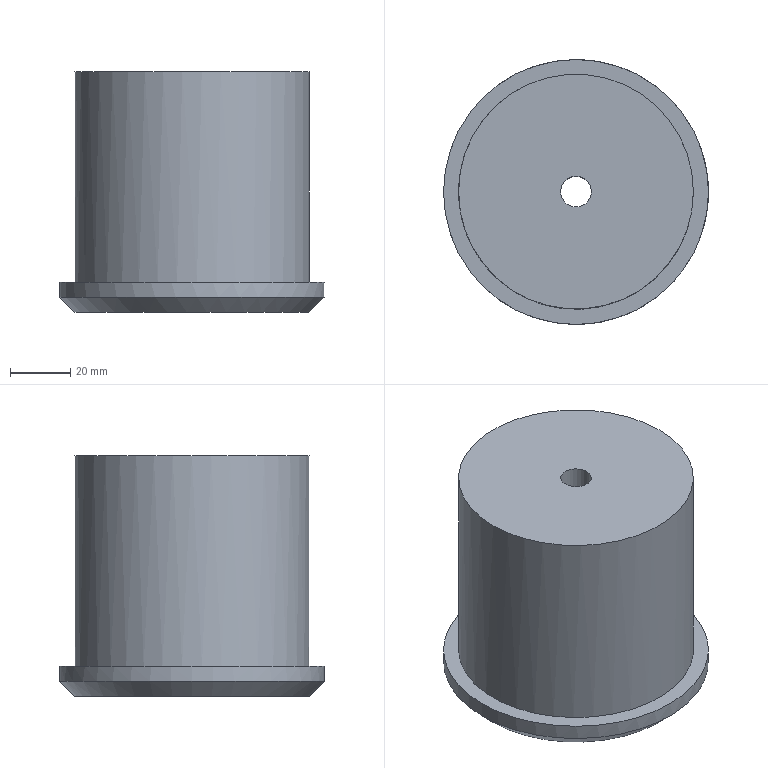Part | STEP file | lll_id810_x_t | 1 solid | 9 faces | box 88 x 88 x 80 mm | volume 376796 mm3 | plane 4 | cylinder 4 | cone 1 | commonest cylinder face diameters 10.2 x1 18.008 x1 78 x1 88 x1
STEP:
#1=CARTESIAN_POINT('',(413.435,500.,-327.5));
#2=VERTEX_POINT('',#1);
#3=CARTESIAN_POINT('',(452.435,500.,-327.5));
#4=DIRECTION('',(0.,0.,-1.));
#5=DIRECTION('',(-1.,0.,0.));
#6=AXIS2_PLACEMENT_3D('',#3,#4,#5);
#7=CIRCLE('',#6,39.);
#8=EDGE_CURVE('',#2,#2,#7,.T.);
#9=ORIENTED_EDGE('',*,*,#8,.F.);
#10=EDGE_LOOP('',(#9));
#11=FACE_BOUND('',#10,.T.);
#12=CARTESIAN_POINT('',(457.535,500.,-327.5));
#13=VERTEX_POINT('',#12);
#14=CARTESIAN_POINT('',(452.435,500.,-327.5));
#15=DIRECTION('',(0.,0.,-1.));
#16=DIRECTION('',(1.,0.,0.));
#17=AXIS2_PLACEMENT_3D('',#14,#15,#16);
#18=CIRCLE('',#17,5.1);
#19=EDGE_CURVE('',#13,#13,#18,.T.);
#20=ORIENTED_EDGE('',*,*,#19,.T.);
#21=EDGE_LOOP('',(#20));
#22=FACE_BOUND('',#21,.T.);
#23=CARTESIAN_POINT('',(452.435,500.,-327.5));
#24=DIRECTION('',(0.,0.,1.));
#25=DIRECTION('',(-1.,0.,0.));
#26=AXIS2_PLACEMENT_3D('',#23,#24,#25);
#27=PLANE('',#26);
#28=ADVANCED_FACE('',(#11,#22),#27,.T.);
#29=CARTESIAN_POINT('',(413.435,500.,-407.5));
#30=VERTEX_POINT('',#29);
#31=CARTESIAN_POINT('',(452.435,500.,-407.5));
#32=DIRECTION('',(0.,0.,-1.));
#33=DIRECTION('',(-1.,0.,0.));
#34=AXIS2_PLACEMENT_3D('',#31,#32,#33);
#35=CIRCLE('',#34,39.);
#36=EDGE_CURVE('',#30,#30,#35,.T.);
#37=ORIENTED_EDGE('',*,*,#36,.T.);
#38=EDGE_LOOP('',(#37));
#39=FACE_BOUND('',#38,.T.);
#40=CARTESIAN_POINT('',(461.439,500.,-407.5));
#41=VERTEX_POINT('',#40);
#42=CARTESIAN_POINT('',(452.435,500.,-407.5));
#43=DIRECTION('',(0.,0.,1.));
#44=DIRECTION('',(1.,0.,0.));
#45=AXIS2_PLACEMENT_3D('',#42,#43,#44);
#46=CIRCLE('',#45,9.004);
#47=EDGE_CURVE('',#41,#41,#46,.T.);
#48=ORIENTED_EDGE('',*,*,#47,.T.);
#49=EDGE_LOOP('',(#48));
#50=FACE_BOUND('',#49,.T.);
#51=CARTESIAN_POINT('',(452.435,500.,-407.5));
#52=DIRECTION('',(0.,0.,-1.));
#53=DIRECTION('',(1.,0.,0.));
#54=AXIS2_PLACEMENT_3D('',#51,#52,#53);
#55=PLANE('',#54);
#56=ADVANCED_FACE('',(#39,#50),#55,.T.);
#57=CARTESIAN_POINT('',(491.435,500.,-397.5));
#58=VERTEX_POINT('',#57);
#59=CARTESIAN_POINT('',(452.435,500.,-397.5));
#60=DIRECTION('',(0.,0.,-1.));
#61=DIRECTION('',(1.,0.,0.));
#62=AXIS2_PLACEMENT_3D('',#59,#60,#61);
#63=CIRCLE('',#62,39.);
#64=EDGE_CURVE('',#58,#58,#63,.T.);
#65=ORIENTED_EDGE('',*,*,#64,.F.);
#66=EDGE_LOOP('',(#65));
#67=FACE_BOUND('',#66,.T.);
#68=ORIENTED_EDGE('',*,*,#8,.T.);
#69=EDGE_LOOP('',(#68));
#70=FACE_BOUND('',#69,.T.);
#71=CARTESIAN_POINT('',(452.435,500.,-327.5));
#72=DIRECTION('',(0.,0.,-1.));
#73=DIRECTION('',(1.,0.,0.));
#74=AXIS2_PLACEMENT_3D('',#71,#72,#73);
#75=CYLINDRICAL_SURFACE('',#74,39.);
#76=ADVANCED_FACE('',(#67,#70),#75,.T.);
#77=ORIENTED_EDGE('',*,*,#64,.T.);
#78=EDGE_LOOP('',(#77));
#79=FACE_BOUND('',#78,.T.);
#80=CARTESIAN_POINT('',(496.435,500.,-397.5));
#81=VERTEX_POINT('',#80);
#82=CARTESIAN_POINT('',(452.435,500.,-397.5));
#83=DIRECTION('',(0.,0.,-1.));
#84=DIRECTION('',(1.,0.,0.));
#85=AXIS2_PLACEMENT_3D('',#82,#83,#84);
#86=CIRCLE('',#85,44.);
#87=EDGE_CURVE('',#81,#81,#86,.T.);
#88=ORIENTED_EDGE('',*,*,#87,.F.);
#89=EDGE_LOOP('',(#88));
#90=FACE_BOUND('',#89,.T.);
#91=CARTESIAN_POINT('',(452.435,500.,-397.5));
#92=DIRECTION('',(0.,0.,1.));
#93=DIRECTION('',(-1.,0.,0.));
#94=AXIS2_PLACEMENT_3D('',#91,#92,#93);
#95=PLANE('',#94);
#96=ADVANCED_FACE('',(#79,#90),#95,.T.);
#97=CARTESIAN_POINT('',(408.435,500.,-402.5));
#98=VERTEX_POINT('',#97);
#99=CARTESIAN_POINT('',(452.435,500.,-402.5));
#100=DIRECTION('',(0.,0.,1.));
#101=DIRECTION('',(-1.,0.,0.));
#102=AXIS2_PLACEMENT_3D('',#99,#100,#101);
#103=CIRCLE('',#102,44.);
#104=EDGE_CURVE('',#98,#98,#103,.T.);
#105=ORIENTED_EDGE('',*,*,#104,.T.);
#106=EDGE_LOOP('',(#105));
#107=FACE_BOUND('',#106,.T.);
#108=ORIENTED_EDGE('',*,*,#87,.T.);
#109=EDGE_LOOP('',(#108));
#110=FACE_BOUND('',#109,.T.);
#111=CARTESIAN_POINT('',(452.435,500.,-407.5));
#112=DIRECTION('',(0.,0.,1.));
#113=DIRECTION('',(-1.,0.,0.));
#114=AXIS2_PLACEMENT_3D('',#111,#112,#113);
#115=CYLINDRICAL_SURFACE('',#114,44.);
#116=ADVANCED_FACE('',(#107,#110),#115,.T.);
#117=ORIENTED_EDGE('',*,*,#36,.F.);
#118=EDGE_LOOP('',(#117));
#119=FACE_BOUND('',#118,.T.);
#120=ORIENTED_EDGE('',*,*,#104,.F.);
#121=EDGE_LOOP('',(#120));
#122=FACE_BOUND('',#121,.T.);
#123=CARTESIAN_POINT('',(452.435,500.,-402.5));
#124=DIRECTION('',(0.,0.,1.));
#125=DIRECTION('',(-1.,0.,0.));
#126=AXIS2_PLACEMENT_3D('',#123,#124,#125);
#127=CONICAL_SURFACE('',#126,44.,45.);
#128=ADVANCED_FACE('',(#119,#122),#127,.T.);
#129=CARTESIAN_POINT('',(457.535,500.,-357.5));
#130=VERTEX_POINT('',#129);
#131=CARTESIAN_POINT('',(452.435,500.,-357.5));
#132=DIRECTION('',(0.,0.,1.));
#133=DIRECTION('',(1.,0.,0.));
#134=AXIS2_PLACEMENT_3D('',#131,#132,#133);
#135=CIRCLE('',#134,5.1);
#136=EDGE_CURVE('',#130,#130,#135,.T.);
#137=ORIENTED_EDGE('',*,*,#136,.F.);
#138=EDGE_LOOP('',(#137));
#139=FACE_BOUND('',#138,.T.);
#140=ORIENTED_EDGE('',*,*,#19,.F.);
#141=EDGE_LOOP('',(#140));
#142=FACE_BOUND('',#141,.T.);
#143=CARTESIAN_POINT('',(452.435,500.,-407.5));
#144=DIRECTION('',(0.,0.,1.));
#145=DIRECTION('',(-1.,0.,0.));
#146=AXIS2_PLACEMENT_3D('',#143,#144,#145);
#147=CYLINDRICAL_SURFACE('',#146,5.1);
#148=ADVANCED_FACE('',(#139,#142),#147,.F.);
#149=ORIENTED_EDGE('',*,*,#136,.T.);
#150=EDGE_LOOP('',(#149));
#151=FACE_BOUND('',#150,.T.);
#152=CARTESIAN_POINT('',(461.439,500.,-357.5));
#153=VERTEX_POINT('',#152);
#154=CARTESIAN_POINT('',(452.435,500.,-357.5));
#155=DIRECTION('',(0.,0.,1.));
#156=DIRECTION('',(1.,0.,0.));
#157=AXIS2_PLACEMENT_3D('',#154,#155,#156);
#158=CIRCLE('',#157,9.004);
#159=EDGE_CURVE('',#153,#153,#158,.T.);
#160=ORIENTED_EDGE('',*,*,#159,.F.);
#161=EDGE_LOOP('',(#160));
#162=FACE_BOUND('',#161,.T.);
#163=CARTESIAN_POINT('',(452.435,500.,-357.5));
#164=DIRECTION('',(0.,0.,1.));
#165=DIRECTION('',(-1.,0.,0.));
#166=AXIS2_PLACEMENT_3D('',#163,#164,#165);
#167=PLANE('',#166);
#168=ADVANCED_FACE('',(#151,#162),#167,.F.);
#169=ORIENTED_EDGE('',*,*,#159,.T.);
#170=EDGE_LOOP('',(#169));
#171=FACE_BOUND('',#170,.T.);
#172=ORIENTED_EDGE('',*,*,#47,.F.);
#173=EDGE_LOOP('',(#172));
#174=FACE_BOUND('',#173,.T.);
#175=CARTESIAN_POINT('',(452.435,500.,-407.5));
#176=DIRECTION('',(0.,0.,1.));
#177=DIRECTION('',(-1.,0.,0.));
#178=AXIS2_PLACEMENT_3D('',#175,#176,#177);
#179=CYLINDRICAL_SURFACE('',#178,9.004);
#180=ADVANCED_FACE('',(#171,#174),#179,.F.);
#181=CLOSED_SHELL('',(#28,#56,#76,#96,#116,#128,#148,#168,#180));
#182=MANIFOLD_SOLID_BREP('',#181);
#183=(LENGTH_UNIT()NAMED_UNIT(*)SI_UNIT(.MILLI.,.METRE.));
#184=UNCERTAINTY_MEASURE_WITH_UNIT(LENGTH_MEASURE(0.00002),#183,'','');
#185=(NAMED_UNIT(*)PLANE_ANGLE_UNIT()SI_UNIT($,.RADIAN.));
#186=PLANE_ANGLE_MEASURE_WITH_UNIT(PLANE_ANGLE_MEASURE(0.01745),#185);
#187=DIMENSIONAL_EXPONENTS(0.,0.,0.,0.,0.,0.,0.);
#188=(CONVERSION_BASED_UNIT('DEGREE',#186)NAMED_UNIT(#187)PLANE_ANGLE_UNIT());
#189=(NAMED_UNIT(*)SI_UNIT($,.STERADIAN.)SOLID_ANGLE_UNIT());
#190=(GEOMETRIC_REPRESENTATION_CONTEXT(3)GLOBAL_UNCERTAINTY_ASSIGNED_CONTEXT((#184))GLOBAL_UNIT_ASSIGNED_CONTEXT((#183,#188,#189))REPRESENTATION_CONTEXT('',''));
#191=ADVANCED_BREP_SHAPE_REPRESENTATION('',(#182),#190);